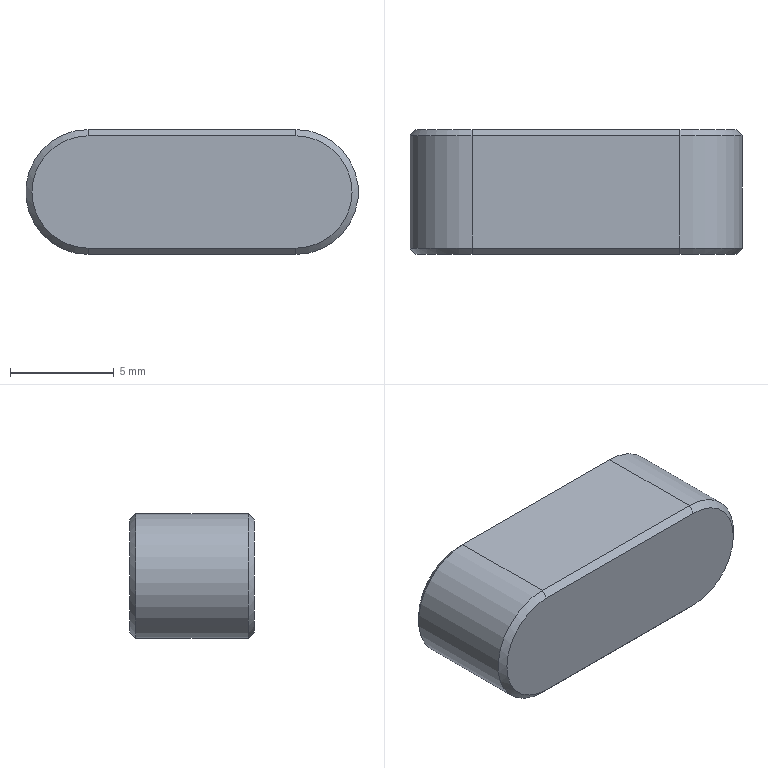Part | NX | features 5003_336_KESS6-16(Default) 2 | 1 solid | 14 faces | box 16 x 6 x 6 mm | volume 526.206 mm3 | plane 8 | cone 4 | cylinder 2 | commonest cylinder face diameters 6 x2
STEP:
#1=CARTESIAN_POINT('',(-5.475,136.2,-144.));
#2=VERTEX_POINT('',#1);
#3=CARTESIAN_POINT('',(-5.475,130.8,-144.));
#4=VERTEX_POINT('',#3);
#5=CARTESIAN_POINT('',(-5.475,130.5,-144.));
#6=DIRECTION('',(0.,1.,0.));
#7=VECTOR('',#6,1000.);
#8=LINE('',#5,#7);
#9=EDGE_CURVE('',#2,#4,#8,.F.);
#10=ORIENTED_EDGE('',*,*,#9,.F.);
#11=CARTESIAN_POINT('',(-5.475,136.2,-150.));
#12=VERTEX_POINT('',#11);
#13=CARTESIAN_POINT('',(-5.475,136.2,-147.));
#14=DIRECTION('',(0.,-1.,0.));
#15=DIRECTION('',(0.,0.,1.));
#16=AXIS2_PLACEMENT_3D('',#13,#14,#15);
#17=CIRCLE('',#16,3.);
#18=EDGE_CURVE('',#2,#12,#17,.T.);
#19=ORIENTED_EDGE('',*,*,#18,.T.);
#20=CARTESIAN_POINT('',(-5.475,130.8,-150.));
#21=VERTEX_POINT('',#20);
#22=CARTESIAN_POINT('',(-5.475,130.5,-150.));
#23=DIRECTION('',(0.,1.,0.));
#24=VECTOR('',#23,1000.);
#25=LINE('',#22,#24);
#26=EDGE_CURVE('',#21,#12,#25,.T.);
#27=ORIENTED_EDGE('',*,*,#26,.F.);
#28=CARTESIAN_POINT('',(-5.475,130.8,-147.));
#29=DIRECTION('',(0.,-1.,0.));
#30=DIRECTION('',(0.,0.,1.));
#31=AXIS2_PLACEMENT_3D('',#28,#29,#30);
#32=CIRCLE('',#31,3.);
#33=EDGE_CURVE('',#21,#4,#32,.F.);
#34=ORIENTED_EDGE('',*,*,#33,.T.);
#35=EDGE_LOOP('',(#10,#19,#27,#34));
#36=FACE_BOUND('',#35,.T.);
#37=CARTESIAN_POINT('',(-5.475,136.5,-147.));
#38=DIRECTION('',(0.,1.,0.));
#39=DIRECTION('',(0.,0.,-1.));
#40=AXIS2_PLACEMENT_3D('',#37,#38,#39);
#41=CYLINDRICAL_SURFACE('',#40,3.);
#42=ADVANCED_FACE('',(#36),#41,.T.);
#43=CARTESIAN_POINT('',(4.525,136.2,-150.));
#44=VERTEX_POINT('',#43);
#45=CARTESIAN_POINT('',(4.525,130.8,-150.));
#46=VERTEX_POINT('',#45);
#47=CARTESIAN_POINT('',(4.525,130.5,-150.));
#48=DIRECTION('',(0.,1.,0.));
#49=VECTOR('',#48,1000.);
#50=LINE('',#47,#49);
#51=EDGE_CURVE('',#44,#46,#50,.F.);
#52=ORIENTED_EDGE('',*,*,#51,.F.);
#53=CARTESIAN_POINT('',(4.525,136.2,-144.));
#54=VERTEX_POINT('',#53);
#55=CARTESIAN_POINT('',(4.525,136.2,-147.));
#56=DIRECTION('',(0.,-1.,0.));
#57=DIRECTION('',(0.,0.,1.));
#58=AXIS2_PLACEMENT_3D('',#55,#56,#57);
#59=CIRCLE('',#58,3.);
#60=EDGE_CURVE('',#44,#54,#59,.T.);
#61=ORIENTED_EDGE('',*,*,#60,.T.);
#62=CARTESIAN_POINT('',(4.525,130.8,-144.));
#63=VERTEX_POINT('',#62);
#64=CARTESIAN_POINT('',(4.525,130.5,-144.));
#65=DIRECTION('',(0.,1.,0.));
#66=VECTOR('',#65,1000.);
#67=LINE('',#64,#66);
#68=EDGE_CURVE('',#63,#54,#67,.T.);
#69=ORIENTED_EDGE('',*,*,#68,.F.);
#70=CARTESIAN_POINT('',(4.525,130.8,-147.));
#71=DIRECTION('',(0.,-1.,0.));
#72=DIRECTION('',(0.,0.,1.));
#73=AXIS2_PLACEMENT_3D('',#70,#71,#72);
#74=CIRCLE('',#73,3.);
#75=EDGE_CURVE('',#63,#46,#74,.F.);
#76=ORIENTED_EDGE('',*,*,#75,.T.);
#77=EDGE_LOOP('',(#52,#61,#69,#76));
#78=FACE_BOUND('',#77,.T.);
#79=CARTESIAN_POINT('',(4.525,130.5,-147.));
#80=DIRECTION('',(0.,1.,0.));
#81=DIRECTION('',(0.,0.,-1.));
#82=AXIS2_PLACEMENT_3D('',#79,#80,#81);
#83=CYLINDRICAL_SURFACE('',#82,3.);
#84=ADVANCED_FACE('',(#78),#83,.T.);
#85=ORIENTED_EDGE('',*,*,#68,.T.);
#86=CARTESIAN_POINT('',(7.525,136.2,-144.));
#87=DIRECTION('',(-1.,0.,0.));
#88=VECTOR('',#87,1000.);
#89=LINE('',#86,#88);
#90=EDGE_CURVE('',#54,#2,#89,.T.);
#91=ORIENTED_EDGE('',*,*,#90,.T.);
#92=ORIENTED_EDGE('',*,*,#9,.T.);
#93=CARTESIAN_POINT('',(4.525,130.8,-144.));
#94=DIRECTION('',(1.,0.,0.));
#95=VECTOR('',#94,1000.);
#96=LINE('',#93,#95);
#97=EDGE_CURVE('',#4,#63,#96,.T.);
#98=ORIENTED_EDGE('',*,*,#97,.T.);
#99=EDGE_LOOP('',(#85,#91,#92,#98));
#100=FACE_BOUND('',#99,.T.);
#101=CARTESIAN_POINT('',(7.525,130.5,-144.));
#102=DIRECTION('',(0.,0.,-1.));
#103=DIRECTION('',(1.,0.,0.));
#104=AXIS2_PLACEMENT_3D('',#101,#102,#103);
#105=PLANE('',#104);
#106=ADVANCED_FACE('',(#100),#105,.F.);
#107=ORIENTED_EDGE('',*,*,#26,.T.);
#108=CARTESIAN_POINT('',(7.525,136.2,-150.));
#109=DIRECTION('',(1.,0.,0.));
#110=VECTOR('',#109,1000.);
#111=LINE('',#108,#110);
#112=EDGE_CURVE('',#12,#44,#111,.T.);
#113=ORIENTED_EDGE('',*,*,#112,.T.);
#114=ORIENTED_EDGE('',*,*,#51,.T.);
#115=CARTESIAN_POINT('',(-5.475,130.8,-150.));
#116=DIRECTION('',(-1.,0.,0.));
#117=VECTOR('',#116,1000.);
#118=LINE('',#115,#117);
#119=EDGE_CURVE('',#46,#21,#118,.T.);
#120=ORIENTED_EDGE('',*,*,#119,.T.);
#121=EDGE_LOOP('',(#107,#113,#114,#120));
#122=FACE_BOUND('',#121,.T.);
#123=CARTESIAN_POINT('',(7.525,130.5,-150.));
#124=DIRECTION('',(0.,0.,1.));
#125=DIRECTION('',(-1.,0.,0.));
#126=AXIS2_PLACEMENT_3D('',#123,#124,#125);
#127=PLANE('',#126);
#128=ADVANCED_FACE('',(#122),#127,.F.);
#129=CARTESIAN_POINT('',(-5.475,130.5,-144.3));
#130=VERTEX_POINT('',#129);
#131=CARTESIAN_POINT('',(-5.475,130.5,-149.7));
#132=VERTEX_POINT('',#131);
#133=CARTESIAN_POINT('',(-5.475,130.5,-147.));
#134=DIRECTION('',(0.,-1.,0.));
#135=DIRECTION('',(0.,0.,1.));
#136=AXIS2_PLACEMENT_3D('',#133,#134,#135);
#137=CIRCLE('',#136,2.7);
#138=EDGE_CURVE('',#130,#132,#137,.T.);
#139=ORIENTED_EDGE('',*,*,#138,.T.);
#140=CARTESIAN_POINT('',(4.525,130.5,-149.7));
#141=VERTEX_POINT('',#140);
#142=CARTESIAN_POINT('',(4.525,130.5,-149.7));
#143=DIRECTION('',(1.,0.,0.));
#144=VECTOR('',#143,1000.);
#145=LINE('',#142,#144);
#146=EDGE_CURVE('',#132,#141,#145,.T.);
#147=ORIENTED_EDGE('',*,*,#146,.T.);
#148=CARTESIAN_POINT('',(4.525,130.5,-144.3));
#149=VERTEX_POINT('',#148);
#150=CARTESIAN_POINT('',(4.525,130.5,-147.));
#151=DIRECTION('',(0.,-1.,0.));
#152=DIRECTION('',(0.,0.,1.));
#153=AXIS2_PLACEMENT_3D('',#150,#151,#152);
#154=CIRCLE('',#153,2.7);
#155=EDGE_CURVE('',#141,#149,#154,.T.);
#156=ORIENTED_EDGE('',*,*,#155,.T.);
#157=CARTESIAN_POINT('',(-5.475,130.5,-144.3));
#158=DIRECTION('',(-1.,0.,0.));
#159=VECTOR('',#158,1000.);
#160=LINE('',#157,#159);
#161=EDGE_CURVE('',#149,#130,#160,.T.);
#162=ORIENTED_EDGE('',*,*,#161,.T.);
#163=EDGE_LOOP('',(#139,#147,#156,#162));
#164=FACE_BOUND('',#163,.T.);
#165=CARTESIAN_POINT('',(-0.475,130.5,-147.));
#166=DIRECTION('',(0.,-1.,0.));
#167=DIRECTION('',(0.,0.,1.));
#168=AXIS2_PLACEMENT_3D('',#165,#166,#167);
#169=PLANE('',#168);
#170=ADVANCED_FACE('',(#164),#169,.T.);
#171=CARTESIAN_POINT('',(4.525,136.5,-144.3));
#172=VERTEX_POINT('',#171);
#173=CARTESIAN_POINT('',(4.525,136.5,-149.7));
#174=VERTEX_POINT('',#173);
#175=CARTESIAN_POINT('',(4.525,136.5,-147.));
#176=DIRECTION('',(0.,-1.,0.));
#177=DIRECTION('',(0.,0.,1.));
#178=AXIS2_PLACEMENT_3D('',#175,#176,#177);
#179=CIRCLE('',#178,2.7);
#180=EDGE_CURVE('',#172,#174,#179,.F.);
#181=ORIENTED_EDGE('',*,*,#180,.T.);
#182=CARTESIAN_POINT('',(-5.475,136.5,-149.7));
#183=VERTEX_POINT('',#182);
#184=CARTESIAN_POINT('',(-0.475,136.5,-149.7));
#185=DIRECTION('',(-1.,0.,0.));
#186=VECTOR('',#185,1000.);
#187=LINE('',#184,#186);
#188=EDGE_CURVE('',#174,#183,#187,.T.);
#189=ORIENTED_EDGE('',*,*,#188,.T.);
#190=CARTESIAN_POINT('',(-5.475,136.5,-144.3));
#191=VERTEX_POINT('',#190);
#192=CARTESIAN_POINT('',(-5.475,136.5,-147.));
#193=DIRECTION('',(0.,-1.,0.));
#194=DIRECTION('',(0.,0.,1.));
#195=AXIS2_PLACEMENT_3D('',#192,#193,#194);
#196=CIRCLE('',#195,2.7);
#197=EDGE_CURVE('',#183,#191,#196,.F.);
#198=ORIENTED_EDGE('',*,*,#197,.T.);
#199=CARTESIAN_POINT('',(-0.475,136.5,-144.3));
#200=DIRECTION('',(1.,0.,0.));
#201=VECTOR('',#200,1000.);
#202=LINE('',#199,#201);
#203=EDGE_CURVE('',#191,#172,#202,.T.);
#204=ORIENTED_EDGE('',*,*,#203,.T.);
#205=EDGE_LOOP('',(#181,#189,#198,#204));
#206=FACE_BOUND('',#205,.T.);
#207=CARTESIAN_POINT('',(-0.475,136.5,-147.));
#208=DIRECTION('',(0.,-1.,0.));
#209=DIRECTION('',(0.,0.,1.));
#210=AXIS2_PLACEMENT_3D('',#207,#208,#209);
#211=PLANE('',#210);
#212=ADVANCED_FACE('',(#206),#211,.F.);
#213=CARTESIAN_POINT('',(4.525,136.5,-144.3));
#214=DIRECTION('',(0.,-0.7071,0.7071));
#215=VECTOR('',#214,1000.);
#216=LINE('',#213,#215);
#217=EDGE_CURVE('',#172,#54,#216,.T.);
#218=ORIENTED_EDGE('',*,*,#217,.F.);
#219=ORIENTED_EDGE('',*,*,#203,.F.);
#220=CARTESIAN_POINT('',(-5.475,136.2,-144.));
#221=DIRECTION('',(0.,0.7071,-0.7071));
#222=VECTOR('',#221,1000.);
#223=LINE('',#220,#222);
#224=EDGE_CURVE('',#2,#191,#223,.T.);
#225=ORIENTED_EDGE('',*,*,#224,.F.);
#226=ORIENTED_EDGE('',*,*,#90,.F.);
#227=EDGE_LOOP('',(#218,#219,#225,#226));
#228=FACE_BOUND('',#227,.T.);
#229=CARTESIAN_POINT('',(7.525,136.2,-144.));
#230=DIRECTION('',(0.,-0.7071,-0.7071));
#231=DIRECTION('',(-1.,0.,0.));
#232=AXIS2_PLACEMENT_3D('',#229,#230,#231);
#233=PLANE('',#232);
#234=ADVANCED_FACE('',(#228),#233,.F.);
#235=ORIENTED_EDGE('',*,*,#224,.T.);
#236=ORIENTED_EDGE('',*,*,#197,.F.);
#237=CARTESIAN_POINT('',(-5.475,136.2,-150.));
#238=DIRECTION('',(0.,0.7071,0.7071));
#239=VECTOR('',#238,1000.);
#240=LINE('',#237,#239);
#241=EDGE_CURVE('',#12,#183,#240,.T.);
#242=ORIENTED_EDGE('',*,*,#241,.F.);
#243=ORIENTED_EDGE('',*,*,#18,.F.);
#244=EDGE_LOOP('',(#235,#236,#242,#243));
#245=FACE_BOUND('',#244,.T.);
#246=CARTESIAN_POINT('',(-5.475,136.5,-147.));
#247=DIRECTION('',(0.,-1.,0.));
#248=DIRECTION('',(0.,0.,1.));
#249=AXIS2_PLACEMENT_3D('',#246,#247,#248);
#250=CONICAL_SURFACE('',#249,2.7,0.7854);
#251=ADVANCED_FACE('',(#245),#250,.T.);
#252=ORIENTED_EDGE('',*,*,#217,.T.);
#253=ORIENTED_EDGE('',*,*,#60,.F.);
#254=CARTESIAN_POINT('',(4.525,136.5,-149.7));
#255=DIRECTION('',(0.,-0.7071,-0.7071));
#256=VECTOR('',#255,1000.);
#257=LINE('',#254,#256);
#258=EDGE_CURVE('',#174,#44,#257,.T.);
#259=ORIENTED_EDGE('',*,*,#258,.F.);
#260=ORIENTED_EDGE('',*,*,#180,.F.);
#261=EDGE_LOOP('',(#252,#253,#259,#260));
#262=FACE_BOUND('',#261,.T.);
#263=CARTESIAN_POINT('',(4.525,136.5,-147.));
#264=DIRECTION('',(0.,-1.,0.));
#265=DIRECTION('',(0.,0.,1.));
#266=AXIS2_PLACEMENT_3D('',#263,#264,#265);
#267=CONICAL_SURFACE('',#266,2.7,0.7854);
#268=ADVANCED_FACE('',(#262),#267,.T.);
#269=ORIENTED_EDGE('',*,*,#241,.T.);
#270=ORIENTED_EDGE('',*,*,#188,.F.);
#271=ORIENTED_EDGE('',*,*,#258,.T.);
#272=ORIENTED_EDGE('',*,*,#112,.F.);
#273=EDGE_LOOP('',(#269,#270,#271,#272));
#274=FACE_BOUND('',#273,.T.);
#275=CARTESIAN_POINT('',(7.525,136.2,-150.));
#276=DIRECTION('',(0.,-0.7071,0.7071));
#277=DIRECTION('',(1.,0.,0.));
#278=AXIS2_PLACEMENT_3D('',#275,#276,#277);
#279=PLANE('',#278);
#280=ADVANCED_FACE('',(#274),#279,.F.);
#281=CARTESIAN_POINT('',(4.525,130.8,-144.));
#282=DIRECTION('',(0.,-0.7071,-0.7071));
#283=VECTOR('',#282,1000.);
#284=LINE('',#281,#283);
#285=EDGE_CURVE('',#63,#149,#284,.T.);
#286=ORIENTED_EDGE('',*,*,#285,.F.);
#287=ORIENTED_EDGE('',*,*,#97,.F.);
#288=CARTESIAN_POINT('',(-5.475,130.5,-144.3));
#289=DIRECTION('',(0.,0.7071,0.7071));
#290=VECTOR('',#289,1000.);
#291=LINE('',#288,#290);
#292=EDGE_CURVE('',#130,#4,#291,.T.);
#293=ORIENTED_EDGE('',*,*,#292,.F.);
#294=ORIENTED_EDGE('',*,*,#161,.F.);
#295=EDGE_LOOP('',(#286,#287,#293,#294));
#296=FACE_BOUND('',#295,.T.);
#297=CARTESIAN_POINT('',(-0.475,130.5,-144.3));
#298=DIRECTION('',(0.,-0.7071,0.7071));
#299=DIRECTION('',(1.,0.,0.));
#300=AXIS2_PLACEMENT_3D('',#297,#298,#299);
#301=PLANE('',#300);
#302=ADVANCED_FACE('',(#296),#301,.T.);
#303=ORIENTED_EDGE('',*,*,#292,.T.);
#304=ORIENTED_EDGE('',*,*,#33,.F.);
#305=CARTESIAN_POINT('',(-5.475,130.5,-149.7));
#306=DIRECTION('',(0.,0.7071,-0.7071));
#307=VECTOR('',#306,1000.);
#308=LINE('',#305,#307);
#309=EDGE_CURVE('',#132,#21,#308,.T.);
#310=ORIENTED_EDGE('',*,*,#309,.F.);
#311=ORIENTED_EDGE('',*,*,#138,.F.);
#312=EDGE_LOOP('',(#303,#304,#310,#311));
#313=FACE_BOUND('',#312,.T.);
#314=CARTESIAN_POINT('',(-5.475,130.5,-147.));
#315=DIRECTION('',(0.,1.,0.));
#316=DIRECTION('',(0.,0.,-1.));
#317=AXIS2_PLACEMENT_3D('',#314,#315,#316);
#318=CONICAL_SURFACE('',#317,2.7,0.7854);
#319=ADVANCED_FACE('',(#313),#318,.T.);
#320=ORIENTED_EDGE('',*,*,#285,.T.);
#321=ORIENTED_EDGE('',*,*,#155,.F.);
#322=CARTESIAN_POINT('',(4.525,130.8,-150.));
#323=DIRECTION('',(0.,-0.7071,0.7071));
#324=VECTOR('',#323,1000.);
#325=LINE('',#322,#324);
#326=EDGE_CURVE('',#46,#141,#325,.T.);
#327=ORIENTED_EDGE('',*,*,#326,.F.);
#328=ORIENTED_EDGE('',*,*,#75,.F.);
#329=EDGE_LOOP('',(#320,#321,#327,#328));
#330=FACE_BOUND('',#329,.T.);
#331=CARTESIAN_POINT('',(4.525,130.5,-147.));
#332=DIRECTION('',(0.,1.,0.));
#333=DIRECTION('',(0.,0.,-1.));
#334=AXIS2_PLACEMENT_3D('',#331,#332,#333);
#335=CONICAL_SURFACE('',#334,2.7,0.7854);
#336=ADVANCED_FACE('',(#330),#335,.T.);
#337=ORIENTED_EDGE('',*,*,#309,.T.);
#338=ORIENTED_EDGE('',*,*,#119,.F.);
#339=ORIENTED_EDGE('',*,*,#326,.T.);
#340=ORIENTED_EDGE('',*,*,#146,.F.);
#341=EDGE_LOOP('',(#337,#338,#339,#340));
#342=FACE_BOUND('',#341,.T.);
#343=CARTESIAN_POINT('',(-0.475,130.5,-149.7));
#344=DIRECTION('',(0.,-0.7071,-0.7071));
#345=DIRECTION('',(-1.,0.,0.));
#346=AXIS2_PLACEMENT_3D('',#343,#344,#345);
#347=PLANE('',#346);
#348=ADVANCED_FACE('',(#342),#347,.T.);
#349=CLOSED_SHELL('',(#42,#84,#106,#128,#170,#212,#234,#251,#268,#280,#302,#319,#336,#348));
#350=MANIFOLD_SOLID_BREP('',#349);
#351=(LENGTH_UNIT()NAMED_UNIT(*)SI_UNIT(.MILLI.,.METRE.));
#352=UNCERTAINTY_MEASURE_WITH_UNIT(LENGTH_MEASURE(0.00001),#351,'','');
#353=(NAMED_UNIT(*)PLANE_ANGLE_UNIT()SI_UNIT($,.RADIAN.));
#354=(NAMED_UNIT(*)SI_UNIT($,.STERADIAN.)SOLID_ANGLE_UNIT());
#355=(GEOMETRIC_REPRESENTATION_CONTEXT(3)GLOBAL_UNCERTAINTY_ASSIGNED_CONTEXT((#352))GLOBAL_UNIT_ASSIGNED_CONTEXT((#351,#353,#354))REPRESENTATION_CONTEXT('',''));
#356=ADVANCED_BREP_SHAPE_REPRESENTATION('',(#350),#355);